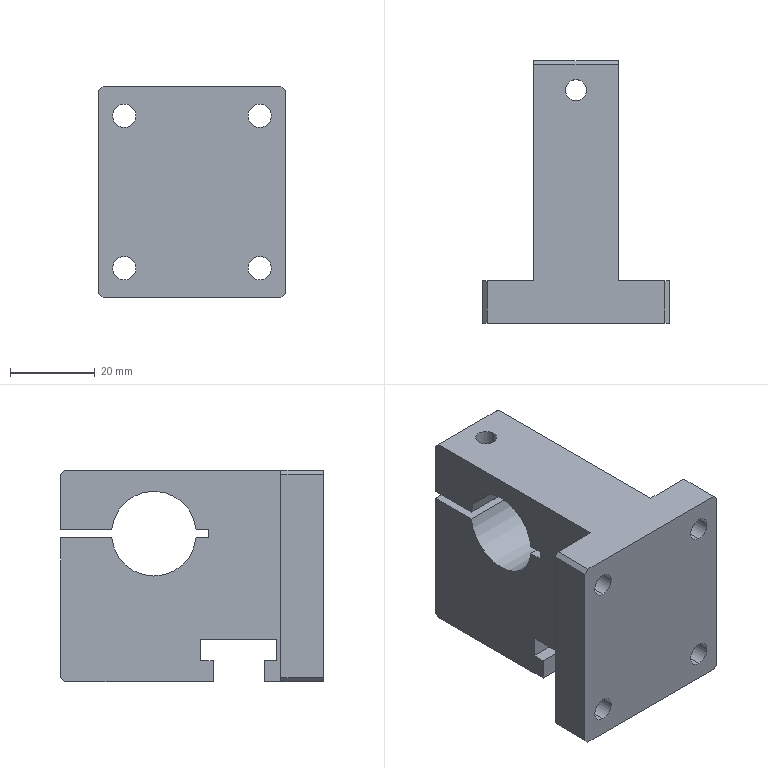Part | SolidWorks | features HoleWzd 2, ICE 2, Chamfer 1, Extrusion 1 | 1 solid | 47 faces | box 44 x 62 x 50 mm | volume 61273 mm3 | plane 31 | cylinder 16 | commonest cylinder face diameters 5.5 x8 5 x2 6.6 x2 11 x2 20 x2
STEP:
#1=CARTESIAN_POINT('',(24.5,55.,50.));
#2=VERTEX_POINT('',#1);
#3=CARTESIAN_POINT('',(19.5,55.,50.));
#4=VERTEX_POINT('',#3);
#5=CARTESIAN_POINT('',(22.,55.,50.));
#6=DIRECTION('',(0.,0.,-1.));
#7=DIRECTION('',(-1.,0.,0.));
#8=AXIS2_PLACEMENT_3D('',#5,#6,#7);
#9=CIRCLE('',#8,2.5);
#10=EDGE_CURVE('',#2,#4,#9,.T.);
#11=ORIENTED_EDGE('',*,*,#10,.F.);
#12=CARTESIAN_POINT('',(24.5,55.,36.));
#13=VERTEX_POINT('',#12);
#14=CARTESIAN_POINT('',(24.5,55.,0.));
#15=DIRECTION('',(0.,0.,-1.));
#16=VECTOR('',#15,1000.);
#17=LINE('',#14,#16);
#18=EDGE_CURVE('',#2,#13,#17,.T.);
#19=ORIENTED_EDGE('',*,*,#18,.T.);
#20=CARTESIAN_POINT('',(19.5,55.,36.));
#21=VERTEX_POINT('',#20);
#22=CARTESIAN_POINT('',(22.,55.,36.));
#23=DIRECTION('',(0.,0.,1.));
#24=DIRECTION('',(1.,0.,0.));
#25=AXIS2_PLACEMENT_3D('',#22,#23,#24);
#26=CIRCLE('',#25,2.5);
#27=EDGE_CURVE('',#21,#13,#26,.T.);
#28=ORIENTED_EDGE('',*,*,#27,.F.);
#29=CARTESIAN_POINT('',(19.5,55.,0.));
#30=DIRECTION('',(0.,0.,-1.));
#31=VECTOR('',#30,1000.);
#32=LINE('',#29,#31);
#33=EDGE_CURVE('',#4,#21,#32,.T.);
#34=ORIENTED_EDGE('',*,*,#33,.F.);
#35=EDGE_LOOP('',(#11,#19,#28,#34));
#36=FACE_OUTER_BOUND('',#35,.T.);
#37=CARTESIAN_POINT('',(22.,55.,0.));
#38=DIRECTION('',(0.,0.,-1.));
#39=DIRECTION('',(-1.,0.,0.));
#40=AXIS2_PLACEMENT_3D('',#37,#38,#39);
#41=CYLINDRICAL_SURFACE('',#40,2.5);
#42=ADVANCED_FACE('',(#36),#41,.F.);
#43=CARTESIAN_POINT('',(27.5,55.,6.8));
#44=VERTEX_POINT('',#43);
#45=CARTESIAN_POINT('',(16.5,55.,6.8));
#46=VERTEX_POINT('',#45);
#47=CARTESIAN_POINT('',(22.,55.,6.8));
#48=DIRECTION('',(0.,0.,-1.));
#49=DIRECTION('',(-1.,0.,0.));
#50=AXIS2_PLACEMENT_3D('',#47,#48,#49);
#51=CIRCLE('',#50,5.5);
#52=EDGE_CURVE('',#44,#46,#51,.T.);
#53=ORIENTED_EDGE('',*,*,#52,.F.);
#54=CARTESIAN_POINT('',(27.5,55.,0.));
#55=VERTEX_POINT('',#54);
#56=CARTESIAN_POINT('',(27.5,55.,0.));
#57=DIRECTION('',(0.,0.,-1.));
#58=VECTOR('',#57,1000.);
#59=LINE('',#56,#58);
#60=EDGE_CURVE('',#44,#55,#59,.T.);
#61=ORIENTED_EDGE('',*,*,#60,.T.);
#62=CARTESIAN_POINT('',(16.5,55.,0.));
#63=VERTEX_POINT('',#62);
#64=CARTESIAN_POINT('',(22.,55.,0.));
#65=DIRECTION('',(0.,0.,-1.));
#66=DIRECTION('',(-1.,0.,0.));
#67=AXIS2_PLACEMENT_3D('',#64,#65,#66);
#68=CIRCLE('',#67,5.5);
#69=EDGE_CURVE('',#55,#63,#68,.T.);
#70=ORIENTED_EDGE('',*,*,#69,.T.);
#71=CARTESIAN_POINT('',(16.5,55.,0.));
#72=DIRECTION('',(0.,0.,-1.));
#73=VECTOR('',#72,1000.);
#74=LINE('',#71,#73);
#75=EDGE_CURVE('',#46,#63,#74,.T.);
#76=ORIENTED_EDGE('',*,*,#75,.F.);
#77=EDGE_LOOP('',(#53,#61,#70,#76));
#78=FACE_OUTER_BOUND('',#77,.T.);
#79=CARTESIAN_POINT('',(22.,55.,0.));
#80=DIRECTION('',(0.,0.,-1.));
#81=DIRECTION('',(-1.,0.,0.));
#82=AXIS2_PLACEMENT_3D('',#79,#80,#81);
#83=CYLINDRICAL_SURFACE('',#82,5.5);
#84=ADVANCED_FACE('',(#78),#83,.F.);
#85=CARTESIAN_POINT('',(25.3,55.,34.));
#86=VERTEX_POINT('',#85);
#87=CARTESIAN_POINT('',(18.7,55.,34.));
#88=VERTEX_POINT('',#87);
#89=CARTESIAN_POINT('',(22.,55.,34.));
#90=DIRECTION('',(0.,0.,-1.));
#91=DIRECTION('',(-1.,0.,0.));
#92=AXIS2_PLACEMENT_3D('',#89,#90,#91);
#93=CIRCLE('',#92,3.3);
#94=EDGE_CURVE('',#86,#88,#93,.T.);
#95=ORIENTED_EDGE('',*,*,#94,.F.);
#96=CARTESIAN_POINT('',(25.3,55.,6.8));
#97=VERTEX_POINT('',#96);
#98=CARTESIAN_POINT('',(25.3,55.,0.));
#99=DIRECTION('',(0.,0.,-1.));
#100=VECTOR('',#99,1000.);
#101=LINE('',#98,#100);
#102=EDGE_CURVE('',#86,#97,#101,.T.);
#103=ORIENTED_EDGE('',*,*,#102,.T.);
#104=CARTESIAN_POINT('',(18.7,55.,6.8));
#105=VERTEX_POINT('',#104);
#106=CARTESIAN_POINT('',(22.,55.,6.8));
#107=DIRECTION('',(0.,0.,-1.));
#108=DIRECTION('',(-1.,0.,0.));
#109=AXIS2_PLACEMENT_3D('',#106,#107,#108);
#110=CIRCLE('',#109,3.3);
#111=EDGE_CURVE('',#97,#105,#110,.T.);
#112=ORIENTED_EDGE('',*,*,#111,.T.);
#113=CARTESIAN_POINT('',(18.7,55.,0.));
#114=DIRECTION('',(0.,0.,-1.));
#115=VECTOR('',#114,1000.);
#116=LINE('',#113,#115);
#117=EDGE_CURVE('',#88,#105,#116,.T.);
#118=ORIENTED_EDGE('',*,*,#117,.F.);
#119=EDGE_LOOP('',(#95,#103,#112,#118));
#120=FACE_OUTER_BOUND('',#119,.T.);
#121=CARTESIAN_POINT('',(22.,55.,0.));
#122=DIRECTION('',(0.,0.,-1.));
#123=DIRECTION('',(-1.,0.,0.));
#124=AXIS2_PLACEMENT_3D('',#121,#122,#123);
#125=CYLINDRICAL_SURFACE('',#124,3.3);
#126=ADVANCED_FACE('',(#120),#125,.F.);
#127=CARTESIAN_POINT('',(38.,10.,4.25));
#128=VERTEX_POINT('',#127);
#129=CARTESIAN_POINT('',(38.,10.,9.75));
#130=VERTEX_POINT('',#129);
#131=CARTESIAN_POINT('',(38.,10.,7.));
#132=DIRECTION('',(0.,1.,0.));
#133=DIRECTION('',(0.,0.,-1.));
#134=AXIS2_PLACEMENT_3D('',#131,#132,#133);
#135=CIRCLE('',#134,2.75);
#136=EDGE_CURVE('',#128,#130,#135,.T.);
#137=ORIENTED_EDGE('',*,*,#136,.T.);
#138=CARTESIAN_POINT('',(38.,0.,9.75));
#139=VERTEX_POINT('',#138);
#140=CARTESIAN_POINT('',(38.,62.001,9.75));
#141=DIRECTION('',(0.,-1.,0.));
#142=VECTOR('',#141,1000.);
#143=LINE('',#140,#142);
#144=EDGE_CURVE('',#130,#139,#143,.T.);
#145=ORIENTED_EDGE('',*,*,#144,.T.);
#146=CARTESIAN_POINT('',(38.,0.,4.25));
#147=VERTEX_POINT('',#146);
#148=CARTESIAN_POINT('',(38.,0.,7.));
#149=DIRECTION('',(0.,-1.,0.));
#150=DIRECTION('',(0.,0.,-1.));
#151=AXIS2_PLACEMENT_3D('',#148,#149,#150);
#152=CIRCLE('',#151,2.75);
#153=EDGE_CURVE('',#139,#147,#152,.T.);
#154=ORIENTED_EDGE('',*,*,#153,.T.);
#155=CARTESIAN_POINT('',(38.,62.001,4.25));
#156=DIRECTION('',(0.,-1.,0.));
#157=VECTOR('',#156,1000.);
#158=LINE('',#155,#157);
#159=EDGE_CURVE('',#128,#147,#158,.T.);
#160=ORIENTED_EDGE('',*,*,#159,.F.);
#161=EDGE_LOOP('',(#137,#145,#154,#160));
#162=FACE_OUTER_BOUND('',#161,.T.);
#163=CARTESIAN_POINT('',(38.,62.001,7.));
#164=DIRECTION('',(0.,-1.,0.));
#165=DIRECTION('',(0.,0.,-1.));
#166=AXIS2_PLACEMENT_3D('',#163,#164,#165);
#167=CYLINDRICAL_SURFACE('',#166,2.75);
#168=ADVANCED_FACE('',(#162),#167,.F.);
#169=CARTESIAN_POINT('',(38.,10.,40.25));
#170=VERTEX_POINT('',#169);
#171=CARTESIAN_POINT('',(38.,10.,45.75));
#172=VERTEX_POINT('',#171);
#173=CARTESIAN_POINT('',(38.,10.,43.));
#174=DIRECTION('',(0.,1.,0.));
#175=DIRECTION('',(0.,0.,-1.));
#176=AXIS2_PLACEMENT_3D('',#173,#174,#175);
#177=CIRCLE('',#176,2.75);
#178=EDGE_CURVE('',#170,#172,#177,.T.);
#179=ORIENTED_EDGE('',*,*,#178,.T.);
#180=CARTESIAN_POINT('',(38.,0.,45.75));
#181=VERTEX_POINT('',#180);
#182=CARTESIAN_POINT('',(38.,62.001,45.75));
#183=DIRECTION('',(0.,-1.,0.));
#184=VECTOR('',#183,1000.);
#185=LINE('',#182,#184);
#186=EDGE_CURVE('',#172,#181,#185,.T.);
#187=ORIENTED_EDGE('',*,*,#186,.T.);
#188=CARTESIAN_POINT('',(38.,0.,40.25));
#189=VERTEX_POINT('',#188);
#190=CARTESIAN_POINT('',(38.,0.,43.));
#191=DIRECTION('',(0.,-1.,0.));
#192=DIRECTION('',(0.,0.,-1.));
#193=AXIS2_PLACEMENT_3D('',#190,#191,#192);
#194=CIRCLE('',#193,2.75);
#195=EDGE_CURVE('',#181,#189,#194,.T.);
#196=ORIENTED_EDGE('',*,*,#195,.T.);
#197=CARTESIAN_POINT('',(38.,62.001,40.25));
#198=DIRECTION('',(0.,-1.,0.));
#199=VECTOR('',#198,1000.);
#200=LINE('',#197,#199);
#201=EDGE_CURVE('',#170,#189,#200,.T.);
#202=ORIENTED_EDGE('',*,*,#201,.F.);
#203=EDGE_LOOP('',(#179,#187,#196,#202));
#204=FACE_OUTER_BOUND('',#203,.T.);
#205=CARTESIAN_POINT('',(38.,62.001,43.));
#206=DIRECTION('',(0.,-1.,0.));
#207=DIRECTION('',(0.,0.,-1.));
#208=AXIS2_PLACEMENT_3D('',#205,#206,#207);
#209=CYLINDRICAL_SURFACE('',#208,2.75);
#210=ADVANCED_FACE('',(#204),#209,.F.);
#211=CARTESIAN_POINT('',(6.,10.,4.25));
#212=VERTEX_POINT('',#211);
#213=CARTESIAN_POINT('',(6.,10.,9.75));
#214=VERTEX_POINT('',#213);
#215=CARTESIAN_POINT('',(6.,10.,7.));
#216=DIRECTION('',(0.,1.,0.));
#217=DIRECTION('',(1.,0.,0.));
#218=AXIS2_PLACEMENT_3D('',#215,#216,#217);
#219=CIRCLE('',#218,2.75);
#220=EDGE_CURVE('',#212,#214,#219,.T.);
#221=ORIENTED_EDGE('',*,*,#220,.T.);
#222=CARTESIAN_POINT('',(6.,0.,9.75));
#223=VERTEX_POINT('',#222);
#224=CARTESIAN_POINT('',(6.,62.001,9.75));
#225=DIRECTION('',(0.,-1.,0.));
#226=VECTOR('',#225,1000.);
#227=LINE('',#224,#226);
#228=EDGE_CURVE('',#214,#223,#227,.T.);
#229=ORIENTED_EDGE('',*,*,#228,.T.);
#230=CARTESIAN_POINT('',(6.,0.,4.25));
#231=VERTEX_POINT('',#230);
#232=CARTESIAN_POINT('',(6.,0.,7.));
#233=DIRECTION('',(0.,-1.,0.));
#234=DIRECTION('',(0.,0.,-1.));
#235=AXIS2_PLACEMENT_3D('',#232,#233,#234);
#236=CIRCLE('',#235,2.75);
#237=EDGE_CURVE('',#223,#231,#236,.T.);
#238=ORIENTED_EDGE('',*,*,#237,.T.);
#239=CARTESIAN_POINT('',(6.,62.001,4.25));
#240=DIRECTION('',(0.,-1.,0.));
#241=VECTOR('',#240,1000.);
#242=LINE('',#239,#241);
#243=EDGE_CURVE('',#212,#231,#242,.T.);
#244=ORIENTED_EDGE('',*,*,#243,.F.);
#245=EDGE_LOOP('',(#221,#229,#238,#244));
#246=FACE_OUTER_BOUND('',#245,.T.);
#247=CARTESIAN_POINT('',(6.,62.001,7.));
#248=DIRECTION('',(0.,-1.,0.));
#249=DIRECTION('',(0.,0.,-1.));
#250=AXIS2_PLACEMENT_3D('',#247,#248,#249);
#251=CYLINDRICAL_SURFACE('',#250,2.75);
#252=ADVANCED_FACE('',(#246),#251,.F.);
#253=CARTESIAN_POINT('',(6.,10.,40.25));
#254=VERTEX_POINT('',#253);
#255=CARTESIAN_POINT('',(6.,10.,45.75));
#256=VERTEX_POINT('',#255);
#257=CARTESIAN_POINT('',(6.,10.,43.));
#258=DIRECTION('',(0.,1.,0.));
#259=DIRECTION('',(1.,0.,0.));
#260=AXIS2_PLACEMENT_3D('',#257,#258,#259);
#261=CIRCLE('',#260,2.75);
#262=EDGE_CURVE('',#254,#256,#261,.T.);
#263=ORIENTED_EDGE('',*,*,#262,.T.);
#264=CARTESIAN_POINT('',(6.,0.,45.75));
#265=VERTEX_POINT('',#264);
#266=CARTESIAN_POINT('',(6.,62.001,45.75));
#267=DIRECTION('',(0.,-1.,0.));
#268=VECTOR('',#267,1000.);
#269=LINE('',#266,#268);
#270=EDGE_CURVE('',#256,#265,#269,.T.);
#271=ORIENTED_EDGE('',*,*,#270,.T.);
#272=CARTESIAN_POINT('',(6.,0.,40.25));
#273=VERTEX_POINT('',#272);
#274=CARTESIAN_POINT('',(6.,0.,43.));
#275=DIRECTION('',(0.,-1.,0.));
#276=DIRECTION('',(0.,0.,-1.));
#277=AXIS2_PLACEMENT_3D('',#274,#275,#276);
#278=CIRCLE('',#277,2.75);
#279=EDGE_CURVE('',#265,#273,#278,.T.);
#280=ORIENTED_EDGE('',*,*,#279,.T.);
#281=CARTESIAN_POINT('',(6.,62.001,40.25));
#282=DIRECTION('',(0.,-1.,0.));
#283=VECTOR('',#282,1000.);
#284=LINE('',#281,#283);
#285=EDGE_CURVE('',#254,#273,#284,.T.);
#286=ORIENTED_EDGE('',*,*,#285,.F.);
#287=EDGE_LOOP('',(#263,#271,#280,#286));
#288=FACE_OUTER_BOUND('',#287,.T.);
#289=CARTESIAN_POINT('',(6.,62.001,43.));
#290=DIRECTION('',(0.,-1.,0.));
#291=DIRECTION('',(0.,0.,-1.));
#292=AXIS2_PLACEMENT_3D('',#289,#290,#291);
#293=CYLINDRICAL_SURFACE('',#292,2.75);
#294=ADVANCED_FACE('',(#288),#293,.F.);
#295=CARTESIAN_POINT('',(22.,55.,0.));
#296=DIRECTION('',(0.,0.,-1.));
#297=DIRECTION('',(-1.,0.,0.));
#298=AXIS2_PLACEMENT_3D('',#295,#296,#297);
#299=CIRCLE('',#298,5.5);
#300=EDGE_CURVE('',#63,#55,#299,.T.);
#301=ORIENTED_EDGE('',*,*,#300,.F.);
#302=ORIENTED_EDGE('',*,*,#69,.F.);
#303=EDGE_LOOP('',(#301,#302));
#304=FACE_BOUND('',#303,.T.);
#305=CARTESIAN_POINT('',(12.,61.,0.));
#306=VERTEX_POINT('',#305);
#307=CARTESIAN_POINT('',(12.,26.,0.));
#308=VERTEX_POINT('',#307);
#309=CARTESIAN_POINT('',(12.,10.,0.));
#310=DIRECTION('',(0.,-1.,0.));
#311=VECTOR('',#310,1000.);
#312=LINE('',#309,#311);
#313=EDGE_CURVE('',#306,#308,#312,.T.);
#314=ORIENTED_EDGE('',*,*,#313,.F.);
#315=CARTESIAN_POINT('',(32.,61.,0.));
#316=VERTEX_POINT('',#315);
#317=CARTESIAN_POINT('',(32.,61.,0.));
#318=DIRECTION('',(1.,0.,0.));
#319=VECTOR('',#318,1000.);
#320=LINE('',#317,#319);
#321=EDGE_CURVE('',#306,#316,#320,.T.);
#322=ORIENTED_EDGE('',*,*,#321,.T.);
#323=CARTESIAN_POINT('',(32.,26.,0.));
#324=VERTEX_POINT('',#323);
#325=CARTESIAN_POINT('',(32.,10.,0.));
#326=DIRECTION('',(0.,1.,0.));
#327=VECTOR('',#326,1000.);
#328=LINE('',#325,#327);
#329=EDGE_CURVE('',#324,#316,#328,.T.);
#330=ORIENTED_EDGE('',*,*,#329,.F.);
#331=CARTESIAN_POINT('',(44.001,26.,0.));
#332=DIRECTION('',(-1.,0.,0.));
#333=VECTOR('',#332,1000.);
#334=LINE('',#331,#333);
#335=EDGE_CURVE('',#324,#308,#334,.T.);
#336=ORIENTED_EDGE('',*,*,#335,.T.);
#337=EDGE_LOOP('',(#314,#322,#330,#336));
#338=FACE_OUTER_BOUND('',#337,.T.);
#339=CARTESIAN_POINT('',(0.,10.,0.));
#340=DIRECTION('',(0.,0.,-1.));
#341=DIRECTION('',(-1.,0.,0.));
#342=AXIS2_PLACEMENT_3D('',#339,#340,#341);
#343=PLANE('',#342);
#344=ADVANCED_FACE('',(#304,#338),#343,.T.);
#345=CARTESIAN_POINT('',(32.,62.,34.));
#346=VERTEX_POINT('',#345);
#347=CARTESIAN_POINT('',(32.,62.,1.));
#348=VERTEX_POINT('',#347);
#349=CARTESIAN_POINT('',(32.,62.,50.));
#350=DIRECTION('',(0.,0.,-1.));
#351=VECTOR('',#350,1000.);
#352=LINE('',#349,#351);
#353=EDGE_CURVE('',#346,#348,#352,.T.);
#354=ORIENTED_EDGE('',*,*,#353,.T.);
#355=CARTESIAN_POINT('',(12.,62.,1.));
#356=VERTEX_POINT('',#355);
#357=CARTESIAN_POINT('',(12.,62.,1.));
#358=DIRECTION('',(-1.,0.,0.));
#359=VECTOR('',#358,1000.);
#360=LINE('',#357,#359);
#361=EDGE_CURVE('',#348,#356,#360,.T.);
#362=ORIENTED_EDGE('',*,*,#361,.T.);
#363=CARTESIAN_POINT('',(12.,62.,34.));
#364=VERTEX_POINT('',#363);
#365=CARTESIAN_POINT('',(12.,62.,50.));
#366=DIRECTION('',(0.,0.,-1.));
#367=VECTOR('',#366,1000.);
#368=LINE('',#365,#367);
#369=EDGE_CURVE('',#364,#356,#368,.T.);
#370=ORIENTED_EDGE('',*,*,#369,.F.);
#371=CARTESIAN_POINT('',(44.001,62.,34.));
#372=DIRECTION('',(-1.,0.,0.));
#373=VECTOR('',#372,1000.);
#374=LINE('',#371,#373);
#375=EDGE_CURVE('',#346,#364,#374,.T.);
#376=ORIENTED_EDGE('',*,*,#375,.F.);
#377=EDGE_LOOP('',(#354,#362,#370,#376));
#378=FACE_OUTER_BOUND('',#377,.T.);
#379=CARTESIAN_POINT('',(12.,62.,50.));
#380=DIRECTION('',(0.,-1.,0.));
#381=DIRECTION('',(0.,0.,-1.));
#382=AXIS2_PLACEMENT_3D('',#379,#380,#381);
#383=PLANE('',#382);
#384=ADVANCED_FACE('',(#378),#383,.F.);
#385=CARTESIAN_POINT('',(0.,10.,49.));
#386=VERTEX_POINT('',#385);
#387=CARTESIAN_POINT('',(0.,10.,1.));
#388=VERTEX_POINT('',#387);
#389=CARTESIAN_POINT('',(0.,10.,50.));
#390=DIRECTION('',(0.,0.,-1.));
#391=VECTOR('',#390,1000.);
#392=LINE('',#389,#391);
#393=EDGE_CURVE('',#386,#388,#392,.T.);
#394=ORIENTED_EDGE('',*,*,#393,.T.);
#395=CARTESIAN_POINT('',(0.,0.,1.));
#396=VERTEX_POINT('',#395);
#397=CARTESIAN_POINT('',(0.,0.,1.));
#398=DIRECTION('',(0.,-1.,0.));
#399=VECTOR('',#398,1000.);
#400=LINE('',#397,#399);
#401=EDGE_CURVE('',#388,#396,#400,.T.);
#402=ORIENTED_EDGE('',*,*,#401,.T.);
#403=CARTESIAN_POINT('',(0.,0.,49.));
#404=VERTEX_POINT('',#403);
#405=CARTESIAN_POINT('',(0.,0.,50.));
#406=DIRECTION('',(0.,0.,-1.));
#407=VECTOR('',#406,1000.);
#408=LINE('',#405,#407);
#409=EDGE_CURVE('',#404,#396,#408,.T.);
#410=ORIENTED_EDGE('',*,*,#409,.F.);
#411=CARTESIAN_POINT('',(0.,0.,49.));
#412=DIRECTION('',(0.,1.,0.));
#413=VECTOR('',#412,1000.);
#414=LINE('',#411,#413);
#415=EDGE_CURVE('',#404,#386,#414,.T.);
#416=ORIENTED_EDGE('',*,*,#415,.T.);
#417=EDGE_LOOP('',(#394,#402,#410,#416));
#418=FACE_OUTER_BOUND('',#417,.T.);
#419=CARTESIAN_POINT('',(0.,0.,50.));
#420=DIRECTION('',(1.,0.,0.));
#421=DIRECTION('',(0.,0.,-1.));
#422=AXIS2_PLACEMENT_3D('',#419,#420,#421);
#423=PLANE('',#422);
#424=ADVANCED_FACE('',(#418),#423,.F.);
#425=CARTESIAN_POINT('',(38.,0.,7.));
#426=DIRECTION('',(0.,-1.,0.));
#427=DIRECTION('',(0.,0.,-1.));
#428=AXIS2_PLACEMENT_3D('',#425,#426,#427);
#429=CIRCLE('',#428,2.75);
#430=EDGE_CURVE('',#147,#139,#429,.T.);
#431=ORIENTED_EDGE('',*,*,#430,.F.);
#432=ORIENTED_EDGE('',*,*,#153,.F.);
#433=EDGE_LOOP('',(#431,#432));
#434=FACE_BOUND('',#433,.T.);
#435=CARTESIAN_POINT('',(38.,0.,43.));
#436=DIRECTION('',(0.,-1.,0.));
#437=DIRECTION('',(0.,0.,-1.));
#438=AXIS2_PLACEMENT_3D('',#435,#436,#437);
#439=CIRCLE('',#438,2.75);
#440=EDGE_CURVE('',#189,#181,#439,.T.);
#441=ORIENTED_EDGE('',*,*,#440,.F.);
#442=ORIENTED_EDGE('',*,*,#195,.F.);
#443=EDGE_LOOP('',(#441,#442));
#444=FACE_BOUND('',#443,.T.);
#445=CARTESIAN_POINT('',(6.,0.,7.));
#446=DIRECTION('',(0.,-1.,0.));
#447=DIRECTION('',(0.,0.,-1.));
#448=AXIS2_PLACEMENT_3D('',#445,#446,#447);
#449=CIRCLE('',#448,2.75);
#450=EDGE_CURVE('',#231,#223,#449,.T.);
#451=ORIENTED_EDGE('',*,*,#450,.F.);
#452=ORIENTED_EDGE('',*,*,#237,.F.);
#453=EDGE_LOOP('',(#451,#452));
#454=FACE_BOUND('',#453,.T.);
#455=CARTESIAN_POINT('',(6.,0.,43.));
#456=DIRECTION('',(0.,-1.,0.));
#457=DIRECTION('',(0.,0.,-1.));
#458=AXIS2_PLACEMENT_3D('',#455,#456,#457);
#459=CIRCLE('',#458,2.75);
#460=EDGE_CURVE('',#273,#265,#459,.T.);
#461=ORIENTED_EDGE('',*,*,#460,.F.);
#462=ORIENTED_EDGE('',*,*,#279,.F.);
#463=EDGE_LOOP('',(#461,#462));
#464=FACE_BOUND('',#463,.T.);
#465=ORIENTED_EDGE('',*,*,#409,.T.);
#466=CARTESIAN_POINT('',(1.,0.,0.));
#467=VERTEX_POINT('',#466);
#468=CARTESIAN_POINT('',(0.,0.,1.));
#469=DIRECTION('',(0.7071,0.,-0.7071));
#470=VECTOR('',#469,1000.);
#471=LINE('',#468,#470);
#472=EDGE_CURVE('',#396,#467,#471,.T.);
#473=ORIENTED_EDGE('',*,*,#472,.T.);
#474=CARTESIAN_POINT('',(43.,0.,0.));
#475=VERTEX_POINT('',#474);
#476=CARTESIAN_POINT('',(0.,0.,0.));
#477=DIRECTION('',(1.,0.,0.));
#478=VECTOR('',#477,1000.);
#479=LINE('',#476,#478);
#480=EDGE_CURVE('',#467,#475,#479,.T.);
#481=ORIENTED_EDGE('',*,*,#480,.T.);
#482=CARTESIAN_POINT('',(44.,0.,1.));
#483=VERTEX_POINT('',#482);
#484=CARTESIAN_POINT('',(44.,0.,1.));
#485=DIRECTION('',(0.7071,0.,0.7071));
#486=VECTOR('',#485,1000.);
#487=LINE('',#484,#486);
#488=EDGE_CURVE('',#475,#483,#487,.T.);
#489=ORIENTED_EDGE('',*,*,#488,.T.);
#490=CARTESIAN_POINT('',(44.,0.,49.));
#491=VERTEX_POINT('',#490);
#492=CARTESIAN_POINT('',(44.,0.,50.));
#493=DIRECTION('',(0.,0.,-1.));
#494=VECTOR('',#493,1000.);
#495=LINE('',#492,#494);
#496=EDGE_CURVE('',#491,#483,#495,.T.);
#497=ORIENTED_EDGE('',*,*,#496,.F.);
#498=CARTESIAN_POINT('',(43.,0.,50.));
#499=VERTEX_POINT('',#498);
#500=CARTESIAN_POINT('',(43.,0.,50.));
#501=DIRECTION('',(-0.7071,0.,0.7071));
#502=VECTOR('',#501,1000.);
#503=LINE('',#500,#502);
#504=EDGE_CURVE('',#491,#499,#503,.T.);
#505=ORIENTED_EDGE('',*,*,#504,.T.);
#506=CARTESIAN_POINT('',(1.,0.,50.));
#507=VERTEX_POINT('',#506);
#508=CARTESIAN_POINT('',(0.,0.,50.));
#509=DIRECTION('',(1.,0.,0.));
#510=VECTOR('',#509,1000.);
#511=LINE('',#508,#510);
#512=EDGE_CURVE('',#507,#499,#511,.T.);
#513=ORIENTED_EDGE('',*,*,#512,.F.);
#514=CARTESIAN_POINT('',(1.,0.,50.));
#515=DIRECTION('',(-0.7071,0.,-0.7071));
#516=VECTOR('',#515,1000.);
#517=LINE('',#514,#516);
#518=EDGE_CURVE('',#507,#404,#517,.T.);
#519=ORIENTED_EDGE('',*,*,#518,.T.);
#520=EDGE_LOOP('',(#465,#473,#481,#489,#497,#505,#513,#519));
#521=FACE_OUTER_BOUND('',#520,.T.);
#522=CARTESIAN_POINT('',(0.,0.,50.));
#523=DIRECTION('',(0.,1.,0.));
#524=DIRECTION('',(0.,0.,1.));
#525=AXIS2_PLACEMENT_3D('',#522,#523,#524);
#526=PLANE('',#525);
#527=ADVANCED_FACE('',(#434,#444,#454,#464,#521),#526,.F.);
#528=CARTESIAN_POINT('',(44.,10.,49.));
#529=VERTEX_POINT('',#528);
#530=CARTESIAN_POINT('',(44.,10.,1.));
#531=VERTEX_POINT('',#530);
#532=CARTESIAN_POINT('',(44.,10.,50.));
#533=DIRECTION('',(0.,0.,-1.));
#534=VECTOR('',#533,1000.);
#535=LINE('',#532,#534);
#536=EDGE_CURVE('',#529,#531,#535,.T.);
#537=ORIENTED_EDGE('',*,*,#536,.F.);
#538=CARTESIAN_POINT('',(44.,0.,49.));
#539=DIRECTION('',(0.,-1.,0.));
#540=VECTOR('',#539,1000.);
#541=LINE('',#538,#540);
#542=EDGE_CURVE('',#529,#491,#541,.T.);
#543=ORIENTED_EDGE('',*,*,#542,.T.);
#544=ORIENTED_EDGE('',*,*,#496,.T.);
#545=CARTESIAN_POINT('',(44.,10.,1.));
#546=DIRECTION('',(0.,1.,0.));
#547=VECTOR('',#546,1000.);
#548=LINE('',#545,#547);
#549=EDGE_CURVE('',#483,#531,#548,.T.);
#550=ORIENTED_EDGE('',*,*,#549,.T.);
#551=EDGE_LOOP('',(#537,#543,#544,#550));
#552=FACE_OUTER_BOUND('',#551,.T.);
#553=CARTESIAN_POINT('',(44.,0.,50.));
#554=DIRECTION('',(-1.,0.,0.));
#555=DIRECTION('',(0.,0.,1.));
#556=AXIS2_PLACEMENT_3D('',#553,#554,#555);
#557=PLANE('',#556);
#558=ADVANCED_FACE('',(#552),#557,.F.);
#559=ORIENTED_EDGE('',*,*,#136,.F.);
#560=CARTESIAN_POINT('',(38.,10.,7.));
#561=DIRECTION('',(0.,1.,0.));
#562=DIRECTION('',(0.,0.,-1.));
#563=AXIS2_PLACEMENT_3D('',#560,#561,#562);
#564=CIRCLE('',#563,2.75);
#565=EDGE_CURVE('',#130,#128,#564,.T.);
#566=ORIENTED_EDGE('',*,*,#565,.F.);
#567=EDGE_LOOP('',(#559,#566));
#568=FACE_BOUND('',#567,.T.);
#569=ORIENTED_EDGE('',*,*,#178,.F.);
#570=CARTESIAN_POINT('',(38.,10.,43.));
#571=DIRECTION('',(0.,1.,0.));
#572=DIRECTION('',(0.,0.,-1.));
#573=AXIS2_PLACEMENT_3D('',#570,#571,#572);
#574=CIRCLE('',#573,2.75);
#575=EDGE_CURVE('',#172,#170,#574,.T.);
#576=ORIENTED_EDGE('',*,*,#575,.F.);
#577=EDGE_LOOP('',(#569,#576));
#578=FACE_BOUND('',#577,.T.);
#579=CARTESIAN_POINT('',(43.,10.,50.));
#580=VERTEX_POINT('',#579);
#581=CARTESIAN_POINT('',(32.,10.,50.));
#582=VERTEX_POINT('',#581);
#583=CARTESIAN_POINT('',(32.,10.,50.));
#584=DIRECTION('',(-1.,0.,0.));
#585=VECTOR('',#584,1000.);
#586=LINE('',#583,#585);
#587=EDGE_CURVE('',#580,#582,#586,.T.);
#588=ORIENTED_EDGE('',*,*,#587,.F.);
#589=CARTESIAN_POINT('',(43.,10.,50.));
#590=DIRECTION('',(0.7071,0.,-0.7071));
#591=VECTOR('',#590,1000.);
#592=LINE('',#589,#591);
#593=EDGE_CURVE('',#580,#529,#592,.T.);
#594=ORIENTED_EDGE('',*,*,#593,.T.);
#595=ORIENTED_EDGE('',*,*,#536,.T.);
#596=CARTESIAN_POINT('',(43.,10.,0.));
#597=VERTEX_POINT('',#596);
#598=CARTESIAN_POINT('',(44.,10.,1.));
#599=DIRECTION('',(-0.7071,0.,-0.7071));
#600=VECTOR('',#599,1000.);
#601=LINE('',#598,#600);
#602=EDGE_CURVE('',#531,#597,#601,.T.);
#603=ORIENTED_EDGE('',*,*,#602,.T.);
#604=CARTESIAN_POINT('',(32.,10.,0.));
#605=VERTEX_POINT('',#604);
#606=CARTESIAN_POINT('',(32.,10.,0.));
#607=DIRECTION('',(-1.,0.,0.));
#608=VECTOR('',#607,1000.);
#609=LINE('',#606,#608);
#610=EDGE_CURVE('',#597,#605,#609,.T.);
#611=ORIENTED_EDGE('',*,*,#610,.T.);
#612=CARTESIAN_POINT('',(32.,10.,50.));
#613=DIRECTION('',(0.,0.,-1.));
#614=VECTOR('',#613,1000.);
#615=LINE('',#612,#614);
#616=EDGE_CURVE('',#582,#605,#615,.T.);
#617=ORIENTED_EDGE('',*,*,#616,.F.);
#618=EDGE_LOOP('',(#588,#594,#595,#603,#611,#617));
#619=FACE_OUTER_BOUND('',#618,.T.);
#620=CARTESIAN_POINT('',(32.,10.,50.));
#621=DIRECTION('',(0.,-1.,0.));
#622=DIRECTION('',(0.,0.,-1.));
#623=AXIS2_PLACEMENT_3D('',#620,#621,#622);
#624=PLANE('',#623);
#625=ADVANCED_FACE('',(#568,#578,#619),#624,.F.);
#626=CARTESIAN_POINT('',(32.,62.,49.));
#627=VERTEX_POINT('',#626);
#628=CARTESIAN_POINT('',(32.,62.,36.));
#629=VERTEX_POINT('',#628);
#630=CARTESIAN_POINT('',(32.,62.,50.));
#631=DIRECTION('',(0.,0.,-1.));
#632=VECTOR('',#631,1000.);
#633=LINE('',#630,#632);
#634=EDGE_CURVE('',#627,#629,#633,.T.);
#635=ORIENTED_EDGE('',*,*,#634,.F.);
#636=CARTESIAN_POINT('',(32.,61.,50.));
#637=VERTEX_POINT('',#636);
#638=CARTESIAN_POINT('',(32.,61.,50.));
#639=DIRECTION('',(0.,-0.7071,0.7071));
#640=VECTOR('',#639,1000.);
#641=LINE('',#638,#640);
#642=EDGE_CURVE('',#627,#637,#641,.T.);
#643=ORIENTED_EDGE('',*,*,#642,.T.);
#644=CARTESIAN_POINT('',(32.,10.,50.));
#645=DIRECTION('',(0.,1.,0.));
#646=VECTOR('',#645,1000.);
#647=LINE('',#644,#646);
#648=EDGE_CURVE('',#582,#637,#647,.T.);
#649=ORIENTED_EDGE('',*,*,#648,.F.);
#650=ORIENTED_EDGE('',*,*,#616,.T.);
#651=CARTESIAN_POINT('',(32.,14.,0.));
#652=VERTEX_POINT('',#651);
#653=CARTESIAN_POINT('',(32.,10.,0.));
#654=DIRECTION('',(0.,1.,0.));
#655=VECTOR('',#654,1000.);
#656=LINE('',#653,#655);
#657=EDGE_CURVE('',#605,#652,#656,.T.);
#658=ORIENTED_EDGE('',*,*,#657,.T.);
#659=CARTESIAN_POINT('',(32.,14.,5.));
#660=VERTEX_POINT('',#659);
#661=CARTESIAN_POINT('',(32.,14.,0.));
#662=DIRECTION('',(0.,0.,-1.));
#663=VECTOR('',#662,1000.);
#664=LINE('',#661,#663);
#665=EDGE_CURVE('',#660,#652,#664,.T.);
#666=ORIENTED_EDGE('',*,*,#665,.F.);
#667=CARTESIAN_POINT('',(32.,11.,5.));
#668=VERTEX_POINT('',#667);
#669=CARTESIAN_POINT('',(32.,11.,5.));
#670=DIRECTION('',(0.,1.,0.));
#671=VECTOR('',#670,1000.);
#672=LINE('',#669,#671);
#673=EDGE_CURVE('',#668,#660,#672,.T.);
#674=ORIENTED_EDGE('',*,*,#673,.F.);
#675=CARTESIAN_POINT('',(32.,11.,10.));
#676=VERTEX_POINT('',#675);
#677=CARTESIAN_POINT('',(32.,11.,5.));
#678=DIRECTION('',(0.,0.,-1.));
#679=VECTOR('',#678,1000.);
#680=LINE('',#677,#679);
#681=EDGE_CURVE('',#676,#668,#680,.T.);
#682=ORIENTED_EDGE('',*,*,#681,.F.);
#683=CARTESIAN_POINT('',(32.,29.,10.));
#684=VERTEX_POINT('',#683);
#685=CARTESIAN_POINT('',(32.,11.,10.));
#686=DIRECTION('',(0.,-1.,0.));
#687=VECTOR('',#686,1000.);
#688=LINE('',#685,#687);
#689=EDGE_CURVE('',#684,#676,#688,.T.);
#690=ORIENTED_EDGE('',*,*,#689,.F.);
#691=CARTESIAN_POINT('',(32.,29.,5.));
#692=VERTEX_POINT('',#691);
#693=CARTESIAN_POINT('',(32.,29.,5.));
#694=DIRECTION('',(0.,0.,1.));
#695=VECTOR('',#694,1000.);
#696=LINE('',#693,#695);
#697=EDGE_CURVE('',#692,#684,#696,.T.);
#698=ORIENTED_EDGE('',*,*,#697,.F.);
#699=CARTESIAN_POINT('',(32.,26.,5.));
#700=VERTEX_POINT('',#699);
#701=CARTESIAN_POINT('',(32.,26.,5.));
#702=DIRECTION('',(0.,1.,0.));
#703=VECTOR('',#702,1000.);
#704=LINE('',#701,#703);
#705=EDGE_CURVE('',#700,#692,#704,.T.);
#706=ORIENTED_EDGE('',*,*,#705,.F.);
#707=CARTESIAN_POINT('',(32.,26.,0.));
#708=DIRECTION('',(0.,0.,1.));
#709=VECTOR('',#708,1000.);
#710=LINE('',#707,#709);
#711=EDGE_CURVE('',#324,#700,#710,.T.);
#712=ORIENTED_EDGE('',*,*,#711,.F.);
#713=ORIENTED_EDGE('',*,*,#329,.T.);
#714=CARTESIAN_POINT('',(32.,62.,1.));
#715=DIRECTION('',(0.,0.7071,0.7071));
#716=VECTOR('',#715,1000.);
#717=LINE('',#714,#716);
#718=EDGE_CURVE('',#316,#348,#717,.T.);
#719=ORIENTED_EDGE('',*,*,#718,.T.);
#720=ORIENTED_EDGE('',*,*,#353,.F.);
#721=CARTESIAN_POINT('',(32.,49.95,34.));
#722=VERTEX_POINT('',#721);
#723=CARTESIAN_POINT('',(32.,49.95,34.));
#724=DIRECTION('',(0.,1.,0.));
#725=VECTOR('',#724,1000.);
#726=LINE('',#723,#725);
#727=EDGE_CURVE('',#722,#346,#726,.T.);
#728=ORIENTED_EDGE('',*,*,#727,.F.);
#729=CARTESIAN_POINT('',(32.,30.05,34.));
#730=VERTEX_POINT('',#729);
#731=CARTESIAN_POINT('',(32.,40.,35.));
#732=DIRECTION('',(1.,0.,0.));
#733=DIRECTION('',(0.,-1.,0.));
#734=AXIS2_PLACEMENT_3D('',#731,#732,#733);
#735=CIRCLE('',#734,10.);
#736=EDGE_CURVE('',#730,#722,#735,.T.);
#737=ORIENTED_EDGE('',*,*,#736,.F.);
#738=CARTESIAN_POINT('',(32.,27.,34.));
#739=VERTEX_POINT('',#738);
#740=CARTESIAN_POINT('',(32.,30.05,34.));
#741=DIRECTION('',(0.,1.,0.));
#742=VECTOR('',#741,1000.);
#743=LINE('',#740,#742);
#744=EDGE_CURVE('',#739,#730,#743,.T.);
#745=ORIENTED_EDGE('',*,*,#744,.F.);
#746=CARTESIAN_POINT('',(32.,27.,36.));
#747=VERTEX_POINT('',#746);
#748=CARTESIAN_POINT('',(32.,27.,34.));
#749=DIRECTION('',(0.,0.,-1.));
#750=VECTOR('',#749,1000.);
#751=LINE('',#748,#750);
#752=EDGE_CURVE('',#747,#739,#751,.T.);
#753=ORIENTED_EDGE('',*,*,#752,.F.);
#754=CARTESIAN_POINT('',(32.,30.05,36.));
#755=VERTEX_POINT('',#754);
#756=CARTESIAN_POINT('',(32.,30.05,36.));
#757=DIRECTION('',(0.,-1.,0.));
#758=VECTOR('',#757,1000.);
#759=LINE('',#756,#758);
#760=EDGE_CURVE('',#755,#747,#759,.T.);
#761=ORIENTED_EDGE('',*,*,#760,.F.);
#762=CARTESIAN_POINT('',(32.,49.95,36.));
#763=VERTEX_POINT('',#762);
#764=CARTESIAN_POINT('',(32.,40.,35.));
#765=DIRECTION('',(1.,0.,0.));
#766=DIRECTION('',(0.,-1.,0.));
#767=AXIS2_PLACEMENT_3D('',#764,#765,#766);
#768=CIRCLE('',#767,10.);
#769=EDGE_CURVE('',#763,#755,#768,.T.);
#770=ORIENTED_EDGE('',*,*,#769,.F.);
#771=CARTESIAN_POINT('',(32.,49.95,36.));
#772=DIRECTION('',(0.,-1.,0.));
#773=VECTOR('',#772,1000.);
#774=LINE('',#771,#773);
#775=EDGE_CURVE('',#629,#763,#774,.T.);
#776=ORIENTED_EDGE('',*,*,#775,.F.);
#777=EDGE_LOOP('',(#635,#643,#649,#650,#658,#666,#674,#682,#690,#698,#706,#712,#713,#719,#720,#728,#737,#745,#753,#761,#770,#776));
#778=FACE_OUTER_BOUND('',#777,.T.);
#779=CARTESIAN_POINT('',(32.,10.,50.));
#780=DIRECTION('',(-1.,0.,0.));
#781=DIRECTION('',(0.,-1.,0.));
#782=AXIS2_PLACEMENT_3D('',#779,#780,#781);
#783=PLANE('',#782);
#784=ADVANCED_FACE('',(#778),#783,.F.);
#785=CARTESIAN_POINT('',(12.,62.,49.));
#786=VERTEX_POINT('',#785);
#787=CARTESIAN_POINT('',(12.,62.,36.));
#788=VERTEX_POINT('',#787);
#789=CARTESIAN_POINT('',(12.,62.,50.));
#790=DIRECTION('',(0.,0.,-1.));
#791=VECTOR('',#790,1000.);
#792=LINE('',#789,#791);
#793=EDGE_CURVE('',#786,#788,#792,.T.);
#794=ORIENTED_EDGE('',*,*,#793,.F.);
#795=CARTESIAN_POINT('',(12.,62.,49.));
#796=DIRECTION('',(1.,0.,0.));
#797=VECTOR('',#796,1000.);
#798=LINE('',#795,#797);
#799=EDGE_CURVE('',#786,#627,#798,.T.);
#800=ORIENTED_EDGE('',*,*,#799,.T.);
#801=ORIENTED_EDGE('',*,*,#634,.T.);
#802=CARTESIAN_POINT('',(44.001,62.,36.));
#803=DIRECTION('',(-1.,0.,0.));
#804=VECTOR('',#803,1000.);
#805=LINE('',#802,#804);
#806=EDGE_CURVE('',#629,#788,#805,.T.);
#807=ORIENTED_EDGE('',*,*,#806,.T.);
#808=EDGE_LOOP('',(#794,#800,#801,#807));
#809=FACE_OUTER_BOUND('',#808,.T.);
#810=CARTESIAN_POINT('',(12.,62.,50.));
#811=DIRECTION('',(0.,-1.,0.));
#812=DIRECTION('',(0.,0.,-1.));
#813=AXIS2_PLACEMENT_3D('',#810,#811,#812);
#814=PLANE('',#813);
#815=ADVANCED_FACE('',(#809),#814,.F.);
#816=CARTESIAN_POINT('',(12.,61.,50.));
#817=VERTEX_POINT('',#816);
#818=CARTESIAN_POINT('',(12.,10.,50.));
#819=VERTEX_POINT('',#818);
#820=CARTESIAN_POINT('',(12.,10.,50.));
#821=DIRECTION('',(0.,-1.,0.));
#822=VECTOR('',#821,1000.);
#823=LINE('',#820,#822);
#824=EDGE_CURVE('',#817,#819,#823,.T.);
#825=ORIENTED_EDGE('',*,*,#824,.F.);
#826=CARTESIAN_POINT('',(12.,61.,50.));
#827=DIRECTION('',(0.,0.7071,-0.7071));
#828=VECTOR('',#827,1000.);
#829=LINE('',#826,#828);
#830=EDGE_CURVE('',#817,#786,#829,.T.);
#831=ORIENTED_EDGE('',*,*,#830,.T.);
#832=ORIENTED_EDGE('',*,*,#793,.T.);
#833=CARTESIAN_POINT('',(12.,49.95,36.));
#834=VERTEX_POINT('',#833);
#835=CARTESIAN_POINT('',(12.,49.95,36.));
#836=DIRECTION('',(0.,1.,0.));
#837=VECTOR('',#836,1000.);
#838=LINE('',#835,#837);
#839=EDGE_CURVE('',#834,#788,#838,.T.);
#840=ORIENTED_EDGE('',*,*,#839,.F.);
#841=CARTESIAN_POINT('',(12.,30.05,36.));
#842=VERTEX_POINT('',#841);
#843=CARTESIAN_POINT('',(12.,40.,35.));
#844=DIRECTION('',(-1.,0.,0.));
#845=DIRECTION('',(0.,-1.,0.));
#846=AXIS2_PLACEMENT_3D('',#843,#844,#845);
#847=CIRCLE('',#846,10.);
#848=EDGE_CURVE('',#842,#834,#847,.T.);
#849=ORIENTED_EDGE('',*,*,#848,.F.);
#850=CARTESIAN_POINT('',(12.,27.,36.));
#851=VERTEX_POINT('',#850);
#852=CARTESIAN_POINT('',(12.,30.05,36.));
#853=DIRECTION('',(0.,1.,0.));
#854=VECTOR('',#853,1000.);
#855=LINE('',#852,#854);
#856=EDGE_CURVE('',#851,#842,#855,.T.);
#857=ORIENTED_EDGE('',*,*,#856,.F.);
#858=CARTESIAN_POINT('',(12.,27.,34.));
#859=VERTEX_POINT('',#858);
#860=CARTESIAN_POINT('',(12.,27.,34.));
#861=DIRECTION('',(0.,0.,1.));
#862=VECTOR('',#861,1000.);
#863=LINE('',#860,#862);
#864=EDGE_CURVE('',#859,#851,#863,.T.);
#865=ORIENTED_EDGE('',*,*,#864,.F.);
#866=CARTESIAN_POINT('',(12.,30.05,34.));
#867=VERTEX_POINT('',#866);
#868=CARTESIAN_POINT('',(12.,30.05,34.));
#869=DIRECTION('',(0.,-1.,0.));
#870=VECTOR('',#869,1000.);
#871=LINE('',#868,#870);
#872=EDGE_CURVE('',#867,#859,#871,.T.);
#873=ORIENTED_EDGE('',*,*,#872,.F.);
#874=CARTESIAN_POINT('',(12.,49.95,34.));
#875=VERTEX_POINT('',#874);
#876=CARTESIAN_POINT('',(12.,40.,35.));
#877=DIRECTION('',(-1.,0.,0.));
#878=DIRECTION('',(0.,-1.,0.));
#879=AXIS2_PLACEMENT_3D('',#876,#877,#878);
#880=CIRCLE('',#879,10.);
#881=EDGE_CURVE('',#875,#867,#880,.T.);
#882=ORIENTED_EDGE('',*,*,#881,.F.);
#883=CARTESIAN_POINT('',(12.,49.95,34.));
#884=DIRECTION('',(0.,-1.,0.));
#885=VECTOR('',#884,1000.);
#886=LINE('',#883,#885);
#887=EDGE_CURVE('',#364,#875,#886,.T.);
#888=ORIENTED_EDGE('',*,*,#887,.F.);
#889=ORIENTED_EDGE('',*,*,#369,.T.);
#890=CARTESIAN_POINT('',(12.,62.,1.));
#891=DIRECTION('',(0.,-0.7071,-0.7071));
#892=VECTOR('',#891,1000.);
#893=LINE('',#890,#892);
#894=EDGE_CURVE('',#356,#306,#893,.T.);
#895=ORIENTED_EDGE('',*,*,#894,.T.);
#896=ORIENTED_EDGE('',*,*,#313,.T.);
#897=CARTESIAN_POINT('',(12.,26.,5.));
#898=VERTEX_POINT('',#897);
#899=CARTESIAN_POINT('',(12.,26.,0.));
#900=DIRECTION('',(0.,0.,-1.));
#901=VECTOR('',#900,1000.);
#902=LINE('',#899,#901);
#903=EDGE_CURVE('',#898,#308,#902,.T.);
#904=ORIENTED_EDGE('',*,*,#903,.F.);
#905=CARTESIAN_POINT('',(12.,29.,5.));
#906=VERTEX_POINT('',#905);
#907=CARTESIAN_POINT('',(12.,26.,5.));
#908=DIRECTION('',(0.,-1.,0.));
#909=VECTOR('',#908,1000.);
#910=LINE('',#907,#909);
#911=EDGE_CURVE('',#906,#898,#910,.T.);
#912=ORIENTED_EDGE('',*,*,#911,.F.);
#913=CARTESIAN_POINT('',(12.,29.,10.));
#914=VERTEX_POINT('',#913);
#915=CARTESIAN_POINT('',(12.,29.,5.));
#916=DIRECTION('',(0.,0.,-1.));
#917=VECTOR('',#916,1000.);
#918=LINE('',#915,#917);
#919=EDGE_CURVE('',#914,#906,#918,.T.);
#920=ORIENTED_EDGE('',*,*,#919,.F.);
#921=CARTESIAN_POINT('',(12.,11.,10.));
#922=VERTEX_POINT('',#921);
#923=CARTESIAN_POINT('',(12.,11.,10.));
#924=DIRECTION('',(0.,1.,0.));
#925=VECTOR('',#924,1000.);
#926=LINE('',#923,#925);
#927=EDGE_CURVE('',#922,#914,#926,.T.);
#928=ORIENTED_EDGE('',*,*,#927,.F.);
#929=CARTESIAN_POINT('',(12.,11.,5.));
#930=VERTEX_POINT('',#929);
#931=CARTESIAN_POINT('',(12.,11.,5.));
#932=DIRECTION('',(0.,0.,1.));
#933=VECTOR('',#932,1000.);
#934=LINE('',#931,#933);
#935=EDGE_CURVE('',#930,#922,#934,.T.);
#936=ORIENTED_EDGE('',*,*,#935,.F.);
#937=CARTESIAN_POINT('',(12.,14.,5.));
#938=VERTEX_POINT('',#937);
#939=CARTESIAN_POINT('',(12.,11.,5.));
#940=DIRECTION('',(0.,-1.,0.));
#941=VECTOR('',#940,1000.);
#942=LINE('',#939,#941);
#943=EDGE_CURVE('',#938,#930,#942,.T.);
#944=ORIENTED_EDGE('',*,*,#943,.F.);
#945=CARTESIAN_POINT('',(12.,14.,0.));
#946=VERTEX_POINT('',#945);
#947=CARTESIAN_POINT('',(12.,14.,0.));
#948=DIRECTION('',(0.,0.,1.));
#949=VECTOR('',#948,1000.);
#950=LINE('',#947,#949);
#951=EDGE_CURVE('',#946,#938,#950,.T.);
#952=ORIENTED_EDGE('',*,*,#951,.F.);
#953=CARTESIAN_POINT('',(12.,10.,0.));
#954=VERTEX_POINT('',#953);
#955=CARTESIAN_POINT('',(12.,10.,0.));
#956=DIRECTION('',(0.,-1.,0.));
#957=VECTOR('',#956,1000.);
#958=LINE('',#955,#957);
#959=EDGE_CURVE('',#946,#954,#958,.T.);
#960=ORIENTED_EDGE('',*,*,#959,.T.);
#961=CARTESIAN_POINT('',(12.,10.,50.));
#962=DIRECTION('',(0.,0.,-1.));
#963=VECTOR('',#962,1000.);
#964=LINE('',#961,#963);
#965=EDGE_CURVE('',#819,#954,#964,.T.);
#966=ORIENTED_EDGE('',*,*,#965,.F.);
#967=EDGE_LOOP('',(#825,#831,#832,#840,#849,#857,#865,#873,#882,#888,#889,#895,#896,#904,#912,#920,#928,#936,#944,#952,#960,#966));
#968=FACE_OUTER_BOUND('',#967,.T.);
#969=CARTESIAN_POINT('',(12.,10.,50.));
#970=DIRECTION('',(1.,0.,0.));
#971=DIRECTION('',(0.,1.,0.));
#972=AXIS2_PLACEMENT_3D('',#969,#970,#971);
#973=PLANE('',#972);
#974=ADVANCED_FACE('',(#968),#973,.F.);
#975=ORIENTED_EDGE('',*,*,#220,.F.);
#976=CARTESIAN_POINT('',(6.,10.,7.));
#977=DIRECTION('',(0.,1.,0.));
#978=DIRECTION('',(1.,0.,0.));
#979=AXIS2_PLACEMENT_3D('',#976,#977,#978);
#980=CIRCLE('',#979,2.75);
#981=EDGE_CURVE('',#214,#212,#980,.T.);
#982=ORIENTED_EDGE('',*,*,#981,.F.);
#983=EDGE_LOOP('',(#975,#982));
#984=FACE_BOUND('',#983,.T.);
#985=ORIENTED_EDGE('',*,*,#262,.F.);
#986=CARTESIAN_POINT('',(6.,10.,43.));
#987=DIRECTION('',(0.,1.,0.));
#988=DIRECTION('',(1.,0.,0.));
#989=AXIS2_PLACEMENT_3D('',#986,#987,#988);
#990=CIRCLE('',#989,2.75);
#991=EDGE_CURVE('',#256,#254,#990,.T.);
#992=ORIENTED_EDGE('',*,*,#991,.F.);
#993=EDGE_LOOP('',(#985,#992));
#994=FACE_BOUND('',#993,.T.);
#995=CARTESIAN_POINT('',(1.,10.,0.));
#996=VERTEX_POINT('',#995);
#997=CARTESIAN_POINT('',(0.,10.,0.));
#998=DIRECTION('',(-1.,0.,0.));
#999=VECTOR('',#998,1000.);
#1000=LINE('',#997,#999);
#1001=EDGE_CURVE('',#954,#996,#1000,.T.);
#1002=ORIENTED_EDGE('',*,*,#1001,.T.);
#1003=CARTESIAN_POINT('',(0.,10.,1.));
#1004=DIRECTION('',(-0.7071,0.,0.7071));
#1005=VECTOR('',#1004,1000.);
#1006=LINE('',#1003,#1005);
#1007=EDGE_CURVE('',#996,#388,#1006,.T.);
#1008=ORIENTED_EDGE('',*,*,#1007,.T.);
#1009=ORIENTED_EDGE('',*,*,#393,.F.);
#1010=CARTESIAN_POINT('',(1.,10.,50.));
#1011=VERTEX_POINT('',#1010);
#1012=CARTESIAN_POINT('',(1.,10.,50.));
#1013=DIRECTION('',(0.7071,0.,0.7071));
#1014=VECTOR('',#1013,1000.);
#1015=LINE('',#1012,#1014);
#1016=EDGE_CURVE('',#386,#1011,#1015,.T.);
#1017=ORIENTED_EDGE('',*,*,#1016,.T.);
#1018=CARTESIAN_POINT('',(0.,10.,50.));
#1019=DIRECTION('',(-1.,0.,0.));
#1020=VECTOR('',#1019,1000.);
#1021=LINE('',#1018,#1020);
#1022=EDGE_CURVE('',#819,#1011,#1021,.T.);
#1023=ORIENTED_EDGE('',*,*,#1022,.F.);
#1024=ORIENTED_EDGE('',*,*,#965,.T.);
#1025=EDGE_LOOP('',(#1002,#1008,#1009,#1017,#1023,#1024));
#1026=FACE_OUTER_BOUND('',#1025,.T.);
#1027=CARTESIAN_POINT('',(0.,10.,50.));
#1028=DIRECTION('',(0.,-1.,0.));
#1029=DIRECTION('',(1.,0.,0.));
#1030=AXIS2_PLACEMENT_3D('',#1027,#1028,#1029);
#1031=PLANE('',#1030);
#1032=ADVANCED_FACE('',(#984,#994,#1026),#1031,.F.);
#1033=CARTESIAN_POINT('',(22.,55.,50.));
#1034=DIRECTION('',(0.,0.,-1.));
#1035=DIRECTION('',(-1.,0.,0.));
#1036=AXIS2_PLACEMENT_3D('',#1033,#1034,#1035);
#1037=CIRCLE('',#1036,2.5);
#1038=EDGE_CURVE('',#4,#2,#1037,.T.);
#1039=ORIENTED_EDGE('',*,*,#1038,.T.);
#1040=ORIENTED_EDGE('',*,*,#10,.T.);
#1041=EDGE_LOOP('',(#1039,#1040));
#1042=FACE_BOUND('',#1041,.T.);
#1043=ORIENTED_EDGE('',*,*,#648,.T.);
#1044=CARTESIAN_POINT('',(0.,61.,50.));
#1045=DIRECTION('',(-1.,0.,0.));
#1046=VECTOR('',#1045,1000.);
#1047=LINE('',#1044,#1046);
#1048=EDGE_CURVE('',#637,#817,#1047,.T.);
#1049=ORIENTED_EDGE('',*,*,#1048,.T.);
#1050=ORIENTED_EDGE('',*,*,#824,.T.);
#1051=ORIENTED_EDGE('',*,*,#1022,.T.);
#1052=CARTESIAN_POINT('',(1.,10.,50.));
#1053=DIRECTION('',(0.,-1.,0.));
#1054=VECTOR('',#1053,1000.);
#1055=LINE('',#1052,#1054);
#1056=EDGE_CURVE('',#1011,#507,#1055,.T.);
#1057=ORIENTED_EDGE('',*,*,#1056,.T.);
#1058=ORIENTED_EDGE('',*,*,#512,.T.);
#1059=CARTESIAN_POINT('',(43.,10.,50.));
#1060=DIRECTION('',(0.,1.,0.));
#1061=VECTOR('',#1060,1000.);
#1062=LINE('',#1059,#1061);
#1063=EDGE_CURVE('',#499,#580,#1062,.T.);
#1064=ORIENTED_EDGE('',*,*,#1063,.T.);
#1065=ORIENTED_EDGE('',*,*,#587,.T.);
#1066=EDGE_LOOP('',(#1043,#1049,#1050,#1051,#1057,#1058,#1064,#1065));
#1067=FACE_OUTER_BOUND('',#1066,.T.);
#1068=CARTESIAN_POINT('',(0.,10.,50.));
#1069=DIRECTION('',(0.,0.,-1.));
#1070=DIRECTION('',(-1.,0.,0.));
#1071=AXIS2_PLACEMENT_3D('',#1068,#1069,#1070);
#1072=PLANE('',#1071);
#1073=ADVANCED_FACE('',(#1042,#1067),#1072,.F.);
#1074=ORIENTED_EDGE('',*,*,#480,.F.);
#1075=CARTESIAN_POINT('',(1.,10.,0.));
#1076=DIRECTION('',(0.,1.,0.));
#1077=VECTOR('',#1076,1000.);
#1078=LINE('',#1075,#1077);
#1079=EDGE_CURVE('',#467,#996,#1078,.T.);
#1080=ORIENTED_EDGE('',*,*,#1079,.T.);
#1081=ORIENTED_EDGE('',*,*,#1001,.F.);
#1082=ORIENTED_EDGE('',*,*,#959,.F.);
#1083=CARTESIAN_POINT('',(44.001,14.,0.));
#1084=DIRECTION('',(-1.,0.,0.));
#1085=VECTOR('',#1084,1000.);
#1086=LINE('',#1083,#1085);
#1087=EDGE_CURVE('',#652,#946,#1086,.T.);
#1088=ORIENTED_EDGE('',*,*,#1087,.F.);
#1089=ORIENTED_EDGE('',*,*,#657,.F.);
#1090=ORIENTED_EDGE('',*,*,#610,.F.);
#1091=CARTESIAN_POINT('',(43.,0.,0.));
#1092=DIRECTION('',(0.,-1.,0.));
#1093=VECTOR('',#1092,1000.);
#1094=LINE('',#1091,#1093);
#1095=EDGE_CURVE('',#597,#475,#1094,.T.);
#1096=ORIENTED_EDGE('',*,*,#1095,.T.);
#1097=EDGE_LOOP('',(#1074,#1080,#1081,#1082,#1088,#1089,#1090,#1096));
#1098=FACE_OUTER_BOUND('',#1097,.T.);
#1099=CARTESIAN_POINT('',(0.,10.,0.));
#1100=DIRECTION('',(0.,0.,-1.));
#1101=DIRECTION('',(-1.,0.,0.));
#1102=AXIS2_PLACEMENT_3D('',#1099,#1100,#1101);
#1103=PLANE('',#1102);
#1104=ADVANCED_FACE('',(#1098),#1103,.T.);
#1105=ORIENTED_EDGE('',*,*,#270,.F.);
#1106=ORIENTED_EDGE('',*,*,#991,.T.);
#1107=ORIENTED_EDGE('',*,*,#285,.T.);
#1108=ORIENTED_EDGE('',*,*,#460,.T.);
#1109=EDGE_LOOP('',(#1105,#1106,#1107,#1108));
#1110=FACE_OUTER_BOUND('',#1109,.T.);
#1111=CARTESIAN_POINT('',(6.,62.001,43.));
#1112=DIRECTION('',(0.,-1.,0.));
#1113=DIRECTION('',(0.,0.,-1.));
#1114=AXIS2_PLACEMENT_3D('',#1111,#1112,#1113);
#1115=CYLINDRICAL_SURFACE('',#1114,2.75);
#1116=ADVANCED_FACE('',(#1110),#1115,.F.);
#1117=ORIENTED_EDGE('',*,*,#228,.F.);
#1118=ORIENTED_EDGE('',*,*,#981,.T.);
#1119=ORIENTED_EDGE('',*,*,#243,.T.);
#1120=ORIENTED_EDGE('',*,*,#450,.T.);
#1121=EDGE_LOOP('',(#1117,#1118,#1119,#1120));
#1122=FACE_OUTER_BOUND('',#1121,.T.);
#1123=CARTESIAN_POINT('',(6.,62.001,7.));
#1124=DIRECTION('',(0.,-1.,0.));
#1125=DIRECTION('',(0.,0.,-1.));
#1126=AXIS2_PLACEMENT_3D('',#1123,#1124,#1125);
#1127=CYLINDRICAL_SURFACE('',#1126,2.75);
#1128=ADVANCED_FACE('',(#1122),#1127,.F.);
#1129=ORIENTED_EDGE('',*,*,#186,.F.);
#1130=ORIENTED_EDGE('',*,*,#575,.T.);
#1131=ORIENTED_EDGE('',*,*,#201,.T.);
#1132=ORIENTED_EDGE('',*,*,#440,.T.);
#1133=EDGE_LOOP('',(#1129,#1130,#1131,#1132));
#1134=FACE_OUTER_BOUND('',#1133,.T.);
#1135=CARTESIAN_POINT('',(38.,62.001,43.));
#1136=DIRECTION('',(0.,-1.,0.));
#1137=DIRECTION('',(0.,0.,-1.));
#1138=AXIS2_PLACEMENT_3D('',#1135,#1136,#1137);
#1139=CYLINDRICAL_SURFACE('',#1138,2.75);
#1140=ADVANCED_FACE('',(#1134),#1139,.F.);
#1141=ORIENTED_EDGE('',*,*,#144,.F.);
#1142=ORIENTED_EDGE('',*,*,#565,.T.);
#1143=ORIENTED_EDGE('',*,*,#159,.T.);
#1144=ORIENTED_EDGE('',*,*,#430,.T.);
#1145=EDGE_LOOP('',(#1141,#1142,#1143,#1144));
#1146=FACE_OUTER_BOUND('',#1145,.T.);
#1147=CARTESIAN_POINT('',(38.,62.001,7.));
#1148=DIRECTION('',(0.,-1.,0.));
#1149=DIRECTION('',(0.,0.,-1.));
#1150=AXIS2_PLACEMENT_3D('',#1147,#1148,#1149);
#1151=CYLINDRICAL_SURFACE('',#1150,2.75);
#1152=ADVANCED_FACE('',(#1146),#1151,.F.);
#1153=ORIENTED_EDGE('',*,*,#736,.T.);
#1154=CARTESIAN_POINT('',(44.001,49.95,34.));
#1155=DIRECTION('',(-1.,0.,0.));
#1156=VECTOR('',#1155,1000.);
#1157=LINE('',#1154,#1156);
#1158=EDGE_CURVE('',#722,#875,#1157,.T.);
#1159=ORIENTED_EDGE('',*,*,#1158,.T.);
#1160=ORIENTED_EDGE('',*,*,#881,.T.);
#1161=CARTESIAN_POINT('',(44.001,30.05,34.));
#1162=DIRECTION('',(-1.,0.,0.));
#1163=VECTOR('',#1162,1000.);
#1164=LINE('',#1161,#1163);
#1165=EDGE_CURVE('',#730,#867,#1164,.T.);
#1166=ORIENTED_EDGE('',*,*,#1165,.F.);
#1167=EDGE_LOOP('',(#1153,#1159,#1160,#1166));
#1168=FACE_OUTER_BOUND('',#1167,.T.);
#1169=CARTESIAN_POINT('',(44.001,40.,35.));
#1170=DIRECTION('',(-1.,0.,0.));
#1171=DIRECTION('',(0.,-1.,0.));
#1172=AXIS2_PLACEMENT_3D('',#1169,#1170,#1171);
#1173=CYLINDRICAL_SURFACE('',#1172,10.);
#1174=ADVANCED_FACE('',(#1168),#1173,.F.);
#1175=CARTESIAN_POINT('',(22.,55.,34.));
#1176=DIRECTION('',(0.,0.,-1.));
#1177=DIRECTION('',(-1.,0.,0.));
#1178=AXIS2_PLACEMENT_3D('',#1175,#1176,#1177);
#1179=CIRCLE('',#1178,3.3);
#1180=EDGE_CURVE('',#88,#86,#1179,.T.);
#1181=ORIENTED_EDGE('',*,*,#1180,.T.);
#1182=ORIENTED_EDGE('',*,*,#94,.T.);
#1183=EDGE_LOOP('',(#1181,#1182));
#1184=FACE_BOUND('',#1183,.T.);
#1185=ORIENTED_EDGE('',*,*,#727,.T.);
#1186=ORIENTED_EDGE('',*,*,#375,.T.);
#1187=ORIENTED_EDGE('',*,*,#887,.T.);
#1188=ORIENTED_EDGE('',*,*,#1158,.F.);
#1189=EDGE_LOOP('',(#1185,#1186,#1187,#1188));
#1190=FACE_OUTER_BOUND('',#1189,.T.);
#1191=CARTESIAN_POINT('',(44.001,49.95,34.));
#1192=DIRECTION('',(0.,0.,-1.));
#1193=DIRECTION('',(-1.,0.,0.));
#1194=AXIS2_PLACEMENT_3D('',#1191,#1192,#1193);
#1195=PLANE('',#1194);
#1196=ADVANCED_FACE('',(#1184,#1190),#1195,.F.);
#1197=ORIENTED_EDGE('',*,*,#27,.T.);
#1198=CARTESIAN_POINT('',(22.,55.,36.));
#1199=DIRECTION('',(0.,0.,1.));
#1200=DIRECTION('',(1.,0.,0.));
#1201=AXIS2_PLACEMENT_3D('',#1198,#1199,#1200);
#1202=CIRCLE('',#1201,2.5);
#1203=EDGE_CURVE('',#13,#21,#1202,.T.);
#1204=ORIENTED_EDGE('',*,*,#1203,.T.);
#1205=EDGE_LOOP('',(#1197,#1204));
#1206=FACE_BOUND('',#1205,.T.);
#1207=ORIENTED_EDGE('',*,*,#775,.T.);
#1208=CARTESIAN_POINT('',(44.001,49.95,36.));
#1209=DIRECTION('',(-1.,0.,0.));
#1210=VECTOR('',#1209,1000.);
#1211=LINE('',#1208,#1210);
#1212=EDGE_CURVE('',#763,#834,#1211,.T.);
#1213=ORIENTED_EDGE('',*,*,#1212,.T.);
#1214=ORIENTED_EDGE('',*,*,#839,.T.);
#1215=ORIENTED_EDGE('',*,*,#806,.F.);
#1216=EDGE_LOOP('',(#1207,#1213,#1214,#1215));
#1217=FACE_OUTER_BOUND('',#1216,.T.);
#1218=CARTESIAN_POINT('',(44.001,49.95,36.));
#1219=DIRECTION('',(0.,0.,1.));
#1220=DIRECTION('',(1.,0.,0.));
#1221=AXIS2_PLACEMENT_3D('',#1218,#1219,#1220);
#1222=PLANE('',#1221);
#1223=ADVANCED_FACE('',(#1206,#1217),#1222,.F.);
#1224=ORIENTED_EDGE('',*,*,#769,.T.);
#1225=CARTESIAN_POINT('',(44.001,30.05,36.));
#1226=DIRECTION('',(-1.,0.,0.));
#1227=VECTOR('',#1226,1000.);
#1228=LINE('',#1225,#1227);
#1229=EDGE_CURVE('',#755,#842,#1228,.T.);
#1230=ORIENTED_EDGE('',*,*,#1229,.T.);
#1231=ORIENTED_EDGE('',*,*,#848,.T.);
#1232=ORIENTED_EDGE('',*,*,#1212,.F.);
#1233=EDGE_LOOP('',(#1224,#1230,#1231,#1232));
#1234=FACE_OUTER_BOUND('',#1233,.T.);
#1235=CARTESIAN_POINT('',(44.001,40.,35.));
#1236=DIRECTION('',(-1.,0.,0.));
#1237=DIRECTION('',(0.,-1.,0.));
#1238=AXIS2_PLACEMENT_3D('',#1235,#1236,#1237);
#1239=CYLINDRICAL_SURFACE('',#1238,10.);
#1240=ADVANCED_FACE('',(#1234),#1239,.F.);
#1241=ORIENTED_EDGE('',*,*,#760,.T.);
#1242=CARTESIAN_POINT('',(44.001,27.,36.));
#1243=DIRECTION('',(-1.,0.,0.));
#1244=VECTOR('',#1243,1000.);
#1245=LINE('',#1242,#1244);
#1246=EDGE_CURVE('',#747,#851,#1245,.T.);
#1247=ORIENTED_EDGE('',*,*,#1246,.T.);
#1248=ORIENTED_EDGE('',*,*,#856,.T.);
#1249=ORIENTED_EDGE('',*,*,#1229,.F.);
#1250=EDGE_LOOP('',(#1241,#1247,#1248,#1249));
#1251=FACE_OUTER_BOUND('',#1250,.T.);
#1252=CARTESIAN_POINT('',(44.001,30.05,36.));
#1253=DIRECTION('',(0.,0.,1.));
#1254=DIRECTION('',(1.,0.,0.));
#1255=AXIS2_PLACEMENT_3D('',#1252,#1253,#1254);
#1256=PLANE('',#1255);
#1257=ADVANCED_FACE('',(#1251),#1256,.F.);
#1258=ORIENTED_EDGE('',*,*,#752,.T.);
#1259=CARTESIAN_POINT('',(44.001,27.,34.));
#1260=DIRECTION('',(-1.,0.,0.));
#1261=VECTOR('',#1260,1000.);
#1262=LINE('',#1259,#1261);
#1263=EDGE_CURVE('',#739,#859,#1262,.T.);
#1264=ORIENTED_EDGE('',*,*,#1263,.T.);
#1265=ORIENTED_EDGE('',*,*,#864,.T.);
#1266=ORIENTED_EDGE('',*,*,#1246,.F.);
#1267=EDGE_LOOP('',(#1258,#1264,#1265,#1266));
#1268=FACE_OUTER_BOUND('',#1267,.T.);
#1269=CARTESIAN_POINT('',(44.001,27.,34.));
#1270=DIRECTION('',(0.,-1.,0.));
#1271=DIRECTION('',(1.,0.,0.));
#1272=AXIS2_PLACEMENT_3D('',#1269,#1270,#1271);
#1273=PLANE('',#1272);
#1274=ADVANCED_FACE('',(#1268),#1273,.F.);
#1275=ORIENTED_EDGE('',*,*,#744,.T.);
#1276=ORIENTED_EDGE('',*,*,#1165,.T.);
#1277=ORIENTED_EDGE('',*,*,#872,.T.);
#1278=ORIENTED_EDGE('',*,*,#1263,.F.);
#1279=EDGE_LOOP('',(#1275,#1276,#1277,#1278));
#1280=FACE_OUTER_BOUND('',#1279,.T.);
#1281=CARTESIAN_POINT('',(44.001,30.05,34.));
#1282=DIRECTION('',(0.,0.,-1.));
#1283=DIRECTION('',(-1.,0.,0.));
#1284=AXIS2_PLACEMENT_3D('',#1281,#1282,#1283);
#1285=PLANE('',#1284);
#1286=ADVANCED_FACE('',(#1280),#1285,.F.);
#1287=ORIENTED_EDGE('',*,*,#711,.T.);
#1288=CARTESIAN_POINT('',(44.001,26.,5.));
#1289=DIRECTION('',(-1.,0.,0.));
#1290=VECTOR('',#1289,1000.);
#1291=LINE('',#1288,#1290);
#1292=EDGE_CURVE('',#700,#898,#1291,.T.);
#1293=ORIENTED_EDGE('',*,*,#1292,.T.);
#1294=ORIENTED_EDGE('',*,*,#903,.T.);
#1295=ORIENTED_EDGE('',*,*,#335,.F.);
#1296=EDGE_LOOP('',(#1287,#1293,#1294,#1295));
#1297=FACE_OUTER_BOUND('',#1296,.T.);
#1298=CARTESIAN_POINT('',(44.001,26.,0.));
#1299=DIRECTION('',(0.,1.,0.));
#1300=DIRECTION('',(-1.,0.,0.));
#1301=AXIS2_PLACEMENT_3D('',#1298,#1299,#1300);
#1302=PLANE('',#1301);
#1303=ADVANCED_FACE('',(#1297),#1302,.F.);
#1304=ORIENTED_EDGE('',*,*,#705,.T.);
#1305=CARTESIAN_POINT('',(44.001,29.,5.));
#1306=DIRECTION('',(-1.,0.,0.));
#1307=VECTOR('',#1306,1000.);
#1308=LINE('',#1305,#1307);
#1309=EDGE_CURVE('',#692,#906,#1308,.T.);
#1310=ORIENTED_EDGE('',*,*,#1309,.T.);
#1311=ORIENTED_EDGE('',*,*,#911,.T.);
#1312=ORIENTED_EDGE('',*,*,#1292,.F.);
#1313=EDGE_LOOP('',(#1304,#1310,#1311,#1312));
#1314=FACE_OUTER_BOUND('',#1313,.T.);
#1315=CARTESIAN_POINT('',(44.001,26.,5.));
#1316=DIRECTION('',(0.,0.,-1.));
#1317=DIRECTION('',(-1.,0.,0.));
#1318=AXIS2_PLACEMENT_3D('',#1315,#1316,#1317);
#1319=PLANE('',#1318);
#1320=ADVANCED_FACE('',(#1314),#1319,.F.);
#1321=ORIENTED_EDGE('',*,*,#697,.T.);
#1322=CARTESIAN_POINT('',(44.001,29.,10.));
#1323=DIRECTION('',(-1.,0.,0.));
#1324=VECTOR('',#1323,1000.);
#1325=LINE('',#1322,#1324);
#1326=EDGE_CURVE('',#684,#914,#1325,.T.);
#1327=ORIENTED_EDGE('',*,*,#1326,.T.);
#1328=ORIENTED_EDGE('',*,*,#919,.T.);
#1329=ORIENTED_EDGE('',*,*,#1309,.F.);
#1330=EDGE_LOOP('',(#1321,#1327,#1328,#1329));
#1331=FACE_OUTER_BOUND('',#1330,.T.);
#1332=CARTESIAN_POINT('',(44.001,29.,5.));
#1333=DIRECTION('',(0.,1.,0.));
#1334=DIRECTION('',(-1.,0.,0.));
#1335=AXIS2_PLACEMENT_3D('',#1332,#1333,#1334);
#1336=PLANE('',#1335);
#1337=ADVANCED_FACE('',(#1331),#1336,.F.);
#1338=ORIENTED_EDGE('',*,*,#689,.T.);
#1339=CARTESIAN_POINT('',(44.001,11.,10.));
#1340=DIRECTION('',(-1.,0.,0.));
#1341=VECTOR('',#1340,1000.);
#1342=LINE('',#1339,#1341);
#1343=EDGE_CURVE('',#676,#922,#1342,.T.);
#1344=ORIENTED_EDGE('',*,*,#1343,.T.);
#1345=ORIENTED_EDGE('',*,*,#927,.T.);
#1346=ORIENTED_EDGE('',*,*,#1326,.F.);
#1347=EDGE_LOOP('',(#1338,#1344,#1345,#1346));
#1348=FACE_OUTER_BOUND('',#1347,.T.);
#1349=CARTESIAN_POINT('',(44.001,11.,10.));
#1350=DIRECTION('',(0.,0.,1.));
#1351=DIRECTION('',(1.,0.,0.));
#1352=AXIS2_PLACEMENT_3D('',#1349,#1350,#1351);
#1353=PLANE('',#1352);
#1354=ADVANCED_FACE('',(#1348),#1353,.F.);
#1355=ORIENTED_EDGE('',*,*,#681,.T.);
#1356=CARTESIAN_POINT('',(44.001,11.,5.));
#1357=DIRECTION('',(-1.,0.,0.));
#1358=VECTOR('',#1357,1000.);
#1359=LINE('',#1356,#1358);
#1360=EDGE_CURVE('',#668,#930,#1359,.T.);
#1361=ORIENTED_EDGE('',*,*,#1360,.T.);
#1362=ORIENTED_EDGE('',*,*,#935,.T.);
#1363=ORIENTED_EDGE('',*,*,#1343,.F.);
#1364=EDGE_LOOP('',(#1355,#1361,#1362,#1363));
#1365=FACE_OUTER_BOUND('',#1364,.T.);
#1366=CARTESIAN_POINT('',(44.001,11.,5.));
#1367=DIRECTION('',(0.,-1.,0.));
#1368=DIRECTION('',(1.,0.,0.));
#1369=AXIS2_PLACEMENT_3D('',#1366,#1367,#1368);
#1370=PLANE('',#1369);
#1371=ADVANCED_FACE('',(#1365),#1370,.F.);
#1372=ORIENTED_EDGE('',*,*,#673,.T.);
#1373=CARTESIAN_POINT('',(44.001,14.,5.));
#1374=DIRECTION('',(-1.,0.,0.));
#1375=VECTOR('',#1374,1000.);
#1376=LINE('',#1373,#1375);
#1377=EDGE_CURVE('',#660,#938,#1376,.T.);
#1378=ORIENTED_EDGE('',*,*,#1377,.T.);
#1379=ORIENTED_EDGE('',*,*,#943,.T.);
#1380=ORIENTED_EDGE('',*,*,#1360,.F.);
#1381=EDGE_LOOP('',(#1372,#1378,#1379,#1380));
#1382=FACE_OUTER_BOUND('',#1381,.T.);
#1383=CARTESIAN_POINT('',(44.001,11.,5.));
#1384=DIRECTION('',(0.,0.,-1.));
#1385=DIRECTION('',(-1.,0.,0.));
#1386=AXIS2_PLACEMENT_3D('',#1383,#1384,#1385);
#1387=PLANE('',#1386);
#1388=ADVANCED_FACE('',(#1382),#1387,.F.);
#1389=ORIENTED_EDGE('',*,*,#665,.T.);
#1390=ORIENTED_EDGE('',*,*,#1087,.T.);
#1391=ORIENTED_EDGE('',*,*,#951,.T.);
#1392=ORIENTED_EDGE('',*,*,#1377,.F.);
#1393=EDGE_LOOP('',(#1389,#1390,#1391,#1392));
#1394=FACE_OUTER_BOUND('',#1393,.T.);
#1395=CARTESIAN_POINT('',(44.001,14.,0.));
#1396=DIRECTION('',(0.,-1.,0.));
#1397=DIRECTION('',(1.,0.,0.));
#1398=AXIS2_PLACEMENT_3D('',#1395,#1396,#1397);
#1399=PLANE('',#1398);
#1400=ADVANCED_FACE('',(#1394),#1399,.F.);
#1401=ORIENTED_EDGE('',*,*,#102,.F.);
#1402=ORIENTED_EDGE('',*,*,#1180,.F.);
#1403=ORIENTED_EDGE('',*,*,#117,.T.);
#1404=CARTESIAN_POINT('',(22.,55.,6.8));
#1405=DIRECTION('',(0.,0.,-1.));
#1406=DIRECTION('',(-1.,0.,0.));
#1407=AXIS2_PLACEMENT_3D('',#1404,#1405,#1406);
#1408=CIRCLE('',#1407,3.3);
#1409=EDGE_CURVE('',#105,#97,#1408,.T.);
#1410=ORIENTED_EDGE('',*,*,#1409,.T.);
#1411=EDGE_LOOP('',(#1401,#1402,#1403,#1410));
#1412=FACE_OUTER_BOUND('',#1411,.T.);
#1413=CARTESIAN_POINT('',(22.,55.,0.));
#1414=DIRECTION('',(0.,0.,-1.));
#1415=DIRECTION('',(-1.,0.,0.));
#1416=AXIS2_PLACEMENT_3D('',#1413,#1414,#1415);
#1417=CYLINDRICAL_SURFACE('',#1416,3.3);
#1418=ADVANCED_FACE('',(#1412),#1417,.F.);
#1419=ORIENTED_EDGE('',*,*,#1409,.F.);
#1420=ORIENTED_EDGE('',*,*,#111,.F.);
#1421=EDGE_LOOP('',(#1419,#1420));
#1422=FACE_BOUND('',#1421,.T.);
#1423=CARTESIAN_POINT('',(22.,55.,6.8));
#1424=DIRECTION('',(0.,0.,-1.));
#1425=DIRECTION('',(-1.,0.,0.));
#1426=AXIS2_PLACEMENT_3D('',#1423,#1424,#1425);
#1427=CIRCLE('',#1426,5.5);
#1428=EDGE_CURVE('',#46,#44,#1427,.T.);
#1429=ORIENTED_EDGE('',*,*,#1428,.T.);
#1430=ORIENTED_EDGE('',*,*,#52,.T.);
#1431=EDGE_LOOP('',(#1429,#1430));
#1432=FACE_OUTER_BOUND('',#1431,.T.);
#1433=CARTESIAN_POINT('',(25.3,55.,6.8));
#1434=DIRECTION('',(0.,0.,1.));
#1435=DIRECTION('',(1.,0.,0.));
#1436=AXIS2_PLACEMENT_3D('',#1433,#1434,#1435);
#1437=PLANE('',#1436);
#1438=ADVANCED_FACE('',(#1422,#1432),#1437,.F.);
#1439=ORIENTED_EDGE('',*,*,#60,.F.);
#1440=ORIENTED_EDGE('',*,*,#1428,.F.);
#1441=ORIENTED_EDGE('',*,*,#75,.T.);
#1442=ORIENTED_EDGE('',*,*,#300,.T.);
#1443=EDGE_LOOP('',(#1439,#1440,#1441,#1442));
#1444=FACE_OUTER_BOUND('',#1443,.T.);
#1445=CARTESIAN_POINT('',(22.,55.,0.));
#1446=DIRECTION('',(0.,0.,-1.));
#1447=DIRECTION('',(-1.,0.,0.));
#1448=AXIS2_PLACEMENT_3D('',#1445,#1446,#1447);
#1449=CYLINDRICAL_SURFACE('',#1448,5.5);
#1450=ADVANCED_FACE('',(#1444),#1449,.F.);
#1451=ORIENTED_EDGE('',*,*,#18,.F.);
#1452=ORIENTED_EDGE('',*,*,#1038,.F.);
#1453=ORIENTED_EDGE('',*,*,#33,.T.);
#1454=ORIENTED_EDGE('',*,*,#1203,.F.);
#1455=EDGE_LOOP('',(#1451,#1452,#1453,#1454));
#1456=FACE_OUTER_BOUND('',#1455,.T.);
#1457=CARTESIAN_POINT('',(22.,55.,0.));
#1458=DIRECTION('',(0.,0.,-1.));
#1459=DIRECTION('',(-1.,0.,0.));
#1460=AXIS2_PLACEMENT_3D('',#1457,#1458,#1459);
#1461=CYLINDRICAL_SURFACE('',#1460,2.5);
#1462=ADVANCED_FACE('',(#1456),#1461,.F.);
#1463=ORIENTED_EDGE('',*,*,#642,.F.);
#1464=ORIENTED_EDGE('',*,*,#799,.F.);
#1465=ORIENTED_EDGE('',*,*,#830,.F.);
#1466=ORIENTED_EDGE('',*,*,#1048,.F.);
#1467=EDGE_LOOP('',(#1463,#1464,#1465,#1466));
#1468=FACE_OUTER_BOUND('',#1467,.T.);
#1469=CARTESIAN_POINT('',(0.,61.,50.));
#1470=DIRECTION('',(0.,-0.7071,-0.7071));
#1471=DIRECTION('',(0.,0.7071,-0.7071));
#1472=AXIS2_PLACEMENT_3D('',#1469,#1470,#1471);
#1473=PLANE('',#1472);
#1474=ADVANCED_FACE('',(#1468),#1473,.F.);
#1475=ORIENTED_EDGE('',*,*,#718,.F.);
#1476=ORIENTED_EDGE('',*,*,#321,.F.);
#1477=ORIENTED_EDGE('',*,*,#894,.F.);
#1478=ORIENTED_EDGE('',*,*,#361,.F.);
#1479=EDGE_LOOP('',(#1475,#1476,#1477,#1478));
#1480=FACE_OUTER_BOUND('',#1479,.T.);
#1481=CARTESIAN_POINT('',(12.,62.,1.));
#1482=DIRECTION('',(0.,0.7071,-0.7071));
#1483=DIRECTION('',(0.,0.7071,0.7071));
#1484=AXIS2_PLACEMENT_3D('',#1481,#1482,#1483);
#1485=PLANE('',#1484);
#1486=ADVANCED_FACE('',(#1480),#1485,.T.);
#1487=ORIENTED_EDGE('',*,*,#1007,.F.);
#1488=ORIENTED_EDGE('',*,*,#1079,.F.);
#1489=ORIENTED_EDGE('',*,*,#472,.F.);
#1490=ORIENTED_EDGE('',*,*,#401,.F.);
#1491=EDGE_LOOP('',(#1487,#1488,#1489,#1490));
#1492=FACE_OUTER_BOUND('',#1491,.T.);
#1493=CARTESIAN_POINT('',(0.,0.,1.));
#1494=DIRECTION('',(-0.7071,0.,-0.7071));
#1495=DIRECTION('',(-0.7071,0.,0.7071));
#1496=AXIS2_PLACEMENT_3D('',#1493,#1494,#1495);
#1497=PLANE('',#1496);
#1498=ADVANCED_FACE('',(#1492),#1497,.T.);
#1499=ORIENTED_EDGE('',*,*,#1016,.F.);
#1500=ORIENTED_EDGE('',*,*,#415,.F.);
#1501=ORIENTED_EDGE('',*,*,#518,.F.);
#1502=ORIENTED_EDGE('',*,*,#1056,.F.);
#1503=EDGE_LOOP('',(#1499,#1500,#1501,#1502));
#1504=FACE_OUTER_BOUND('',#1503,.T.);
#1505=CARTESIAN_POINT('',(1.,10.,50.));
#1506=DIRECTION('',(0.7071,0.,-0.7071));
#1507=DIRECTION('',(-0.7071,0.,-0.7071));
#1508=AXIS2_PLACEMENT_3D('',#1505,#1506,#1507);
#1509=PLANE('',#1508);
#1510=ADVANCED_FACE('',(#1504),#1509,.F.);
#1511=ORIENTED_EDGE('',*,*,#504,.F.);
#1512=ORIENTED_EDGE('',*,*,#542,.F.);
#1513=ORIENTED_EDGE('',*,*,#593,.F.);
#1514=ORIENTED_EDGE('',*,*,#1063,.F.);
#1515=EDGE_LOOP('',(#1511,#1512,#1513,#1514));
#1516=FACE_OUTER_BOUND('',#1515,.T.);
#1517=CARTESIAN_POINT('',(43.,10.,50.));
#1518=DIRECTION('',(-0.7071,0.,-0.7071));
#1519=DIRECTION('',(-0.7071,0.,0.7071));
#1520=AXIS2_PLACEMENT_3D('',#1517,#1518,#1519);
#1521=PLANE('',#1520);
#1522=ADVANCED_FACE('',(#1516),#1521,.F.);
#1523=ORIENTED_EDGE('',*,*,#488,.F.);
#1524=ORIENTED_EDGE('',*,*,#1095,.F.);
#1525=ORIENTED_EDGE('',*,*,#602,.F.);
#1526=ORIENTED_EDGE('',*,*,#549,.F.);
#1527=EDGE_LOOP('',(#1523,#1524,#1525,#1526));
#1528=FACE_OUTER_BOUND('',#1527,.T.);
#1529=CARTESIAN_POINT('',(44.,0.,1.));
#1530=DIRECTION('',(0.7071,0.,-0.7071));
#1531=DIRECTION('',(-0.7071,0.,-0.7071));
#1532=AXIS2_PLACEMENT_3D('',#1529,#1530,#1531);
#1533=PLANE('',#1532);
#1534=ADVANCED_FACE('',(#1528),#1533,.T.);
#1535=CLOSED_SHELL('',(#42,#84,#126,#168,#210,#252,#294,#344,#384,#424,#527,#558,#625,#784,#815,#974,#1032,#1073,#1104,#1116,#1128,#1140,#1152,#1174,#1196,#1223,#1240,#1257,#1274,#1286,#1303,#1320,#1337,#1354,#1371,#1388,#1400,#1418,#1438,#1450,#1462,#1474,#1486,#1498,#1510,#1522,#1534));
#1536=MANIFOLD_SOLID_BREP('',#1535);
#1537=CARTESIAN_POINT('',(0.,0.,0.));
#1538=DIRECTION('',(0.,0.,1.));
#1539=DIRECTION('',(1.,0.,0.));
#1540=AXIS2_PLACEMENT_3D('',#1537,#1538,#1539);
#1541=(LENGTH_UNIT()NAMED_UNIT(*)SI_UNIT(.MILLI.,.METRE.));
#1542=UNCERTAINTY_MEASURE_WITH_UNIT(LENGTH_MEASURE(0.00001),#1541,'','');
#1543=(NAMED_UNIT(*)PLANE_ANGLE_UNIT()SI_UNIT($,.RADIAN.));
#1544=(NAMED_UNIT(*)SI_UNIT($,.STERADIAN.)SOLID_ANGLE_UNIT());
#1545=(GEOMETRIC_REPRESENTATION_CONTEXT(3)GLOBAL_UNCERTAINTY_ASSIGNED_CONTEXT((#1542))GLOBAL_UNIT_ASSIGNED_CONTEXT((#1541,#1543,#1544))REPRESENTATION_CONTEXT('',''));
#1546=ADVANCED_BREP_SHAPE_REPRESENTATION('',(#1536,#1540),#1545);